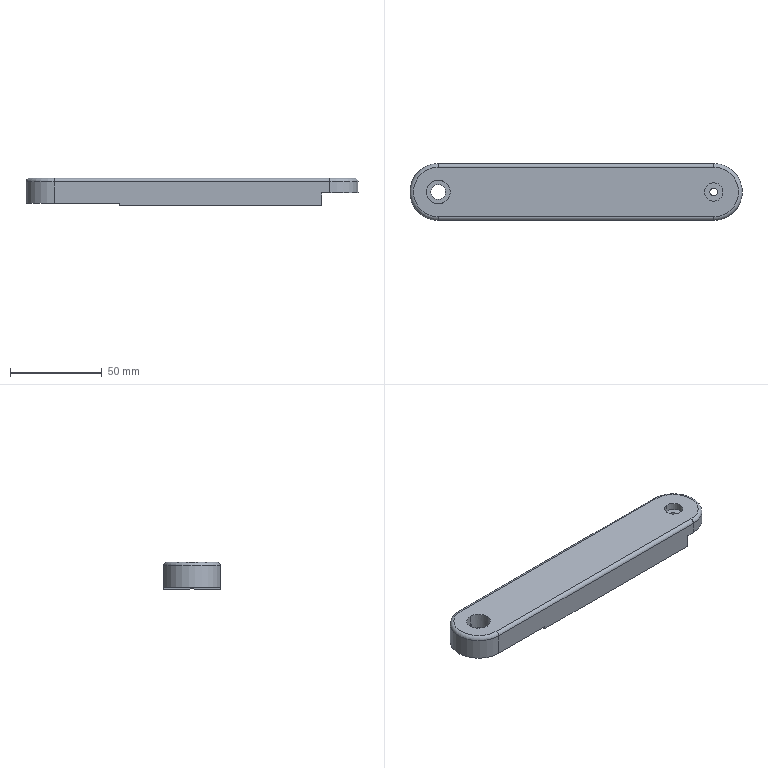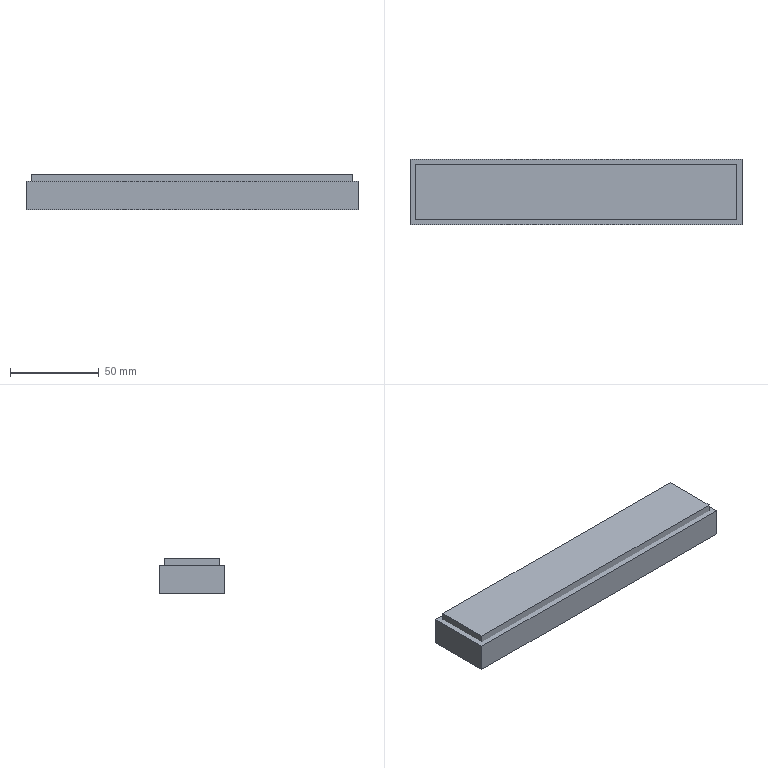CAM job | NX | 3-axis milling, drilling | part box 181 x 31 x 15 mm | stock box 187 x 37 x 20 mm
Tools:
number,name,description,diameter,corner_radius,flute_length,length,flutes
19,D80,Milling Tool-5 Parameters,80.0,0.0,50.0,75.0,2
1,D6A45,Milling Tool-5 Parameters,6.0,0.0,50.0,75.0,2
2,2.1ZT,Drilling Tool,2.05,0.0,35.0,50.0,2
16,1.6ZT,Drilling Tool,1.6,0.0,35.0,50.0,2
24,1.5ZT,Drilling Tool,1.5,0.0,35.0,50.0,2
4,4.2ZT,Drilling Tool,4.2,0.0,35.0,50.0,2
15,D10,Milling Tool-5 Parameters,10.0,0.0,50.0,75.0,2
14,D10JING,Milling Tool-5 Parameters,10.0,0.0,50.0,75.0,2
12,D6,Milling Tool-5 Parameters,6.0,0.0,50.0,75.0,2
17,D2,Milling Tool-5 Parameters,2.0,0.0,50.0,75.0,2
11,D4,Milling Tool-5 Parameters,4.0,0.0,50.0,75.0,2
21,R2,Milling Tool-5 Parameters,4.0,2.0,50.0,75.0,2
18,D6R0.5,Milling Tool-5 Parameters,6.0,0.5,50.0,75.0,2
Operations:
program,operation,operation_type,tool,method,geometry_group,spindle_rpm,surface_speed,feed_per_tooth,feed_cut,feed_plunge,cut_length_mm,path_length_mm,cut_time_min,machine_time_min
1,FLOOR_WALL_COPY,VolumeBased25DMillingOperation,D80,METHOD,A,6500.0,1633.0,0.1154,1500.0,100.0,283.0,337.0,0.1887,0.1941
1,DRILLING_COPY_1,Operation,D6A45,METHOD,A,5000.0,94.0,0.035,350.0,0.0,32.0,352.12,0.0914,0.1234
1,DRILLING_COPY_1_COPY,Operation,2.1ZT,METHOD,A,2000.0,12.0,0.0375,150.0,0.0,33.232,147.712,0.2215,0.233
1,DRILLING_COPY_1_COPY_COPY,Operation,1.6ZT,METHOD,A,2000.0,12.0,0.0375,150.0,0.0,39.923,210.521,0.2662,0.2832
1,DRILLING_COPY_1_COPY_COPY_COPY,Operation,1.5ZT,METHOD,A,2000.0,12.0,0.0375,150.0,0.0,51.003,232.681,0.34,0.3582
1,DRILLING_COPY_1_COPY_1,Operation,4.2ZT,METHOD,A,2000.0,34.0,0.05,200.0,0.0,20.262,100.524,0.1013,0.1093
1,ADAPTIVE_MILLING,CavityMilling,D10,METHOD,A,9500.0,298.0,0.1579,3000.0,1000.0,1947.53,2284.173,0.6532,0.6868
1,FLOOR_WALL,VolumeBased25DMillingOperation,D10,METHOD,A,9500.0,298.0,0.1316,2500.0,1000.0,1273.37,1440.847,0.5474,0.5641
1,FLOOR_WALL_COPY_1,VolumeBased25DMillingOperation,D10,METHOD,A,9500.0,298.0,0.1316,2500.0,1000.0,747.315,828.738,0.3098,0.318
1,ZLEVEL_PROFILE_COPY_1_COPY_COPY_1,ZLevelMilling,D10JING,METHOD,A,9500.0,298.0,0.0632,1200.0,1000.0,436.29,524.29,0.3642,0.373
1,FLOOR_WALL_1,VolumeBased25DMillingOperation,D10JING,METHOD,A,9500.0,298.0,0.0658,1250.0,100.0,676.572,1136.641,0.5413,0.5873
1,FLOOR_WALL_COPY_1_COPY,VolumeBased25DMillingOperation,D6,METHOD,A,9500.0,179.0,0.0868,1650.0,1000.0,1172.176,1259.534,0.7661,0.7748
1,FLOOR_WALL_1_COPY,VolumeBased25DMillingOperation,D6,METHOD,A,9500.0,298.0,0.0658,1250.0,100.0,364.716,558.998,0.2918,0.3112
1,HOLE_MILLING,CylinderMilling,D6,METHOD,A,9500.0,0.0,0.0,1650.0,100.0,270.469,431.069,0.1639,0.18
1,HOLE_MILLING_COPY,CylinderMilling,D4,METHOD,A,9500.0,0.0,0.0,1650.0,100.0,583.153,658.953,0.3534,0.361
1,ZLEVEL_PROFILE,ZLevelMilling,D2,METHOD,A,9500.0,59.0,0.0579,1100.0,100.0,348.462,844.207,0.3168,0.3664
1,FIXED_CONTOUR,SurfaceContour,R2,METHOD,A,9500.0,119.0,0.1316,2500.0,1000.0,1156.287,1209.887,0.465,0.4704
1,PLANAR_MILL_COPY_COPY_COPY_COPY_COPY_COPY_1_COPY_1,PlanarMilling,D6A45,METHOD,A,9500.0,179.0,0.0658,1250.0,100.0,298.924,357.924,0.2391,0.245
1,PLANAR_MILL_COPY_COPY_COPY_COPY_COPY_COPY_1_COPY_1_COPY,PlanarMilling,D6A45,METHOD,A,9500.0,179.0,0.0658,1250.0,100.0,92.815,413.435,0.0743,0.1063
1,PLANAR_MILL_COPY_COPY_COPY_COPY_COPY_COPY_1_COPY_1_COPY_COPY,PlanarMilling,D6A45,METHOD,A,9500.0,179.0,0.0658,1250.0,100.0,277.061,506.146,0.2216,0.2446
1,DRILLING_COPY_1_COPY_2,Operation,D6A45,METHOD,A,5000.0,94.0,0.035,350.0,0.0,28.35,337.279,0.081,0.1119
1,刀补11,CylinderMilling,D4,METHOD,A,9500.0,0.0,0.0526,1000.0,100.0,106.559,182.359,0.1066,0.1141
1,刀补12,CylinderMilling,D6,METHOD,A,9500.0,0.0,0.0526,1000.0,100.0,90.078,250.678,0.0901,0.1061
2,FLOOR_WALL_COPY_COPY,VolumeBased25DMillingOperation,D80,METHOD,B,6500.0,1633.0,0.1154,1500.0,100.0,1385.0,2719.001,0.9233,1.057
2,HOLE_MILLING_COPY_1,CylinderMilling,D6,METHOD,B,9500.0,0.0,0.0,1650.0,100.0,438.049,506.549,0.2655,0.2723
2,HOLE_MILLING_COPY_COPY,CylinderMilling,D4,METHOD,B,9500.0,0.0,0.0,1650.0,100.0,466.634,534.634,0.2828,0.2896
2,PLANAR_MILL_COPY_COPY_COPY_COPY_COPY_COPY_1_COPY_1_COPY_1,PlanarMilling,D6A45,METHOD,B,9500.0,179.0,0.0658,1250.0,100.0,77.073,347.985,0.0617,0.0887
2,ZLEVEL_PROFILE_1,ZLevelMilling,D6R0.5,METHOD,B,9500.0,119.0,0.1842,3500.0,100.0,15642.139,15698.648,4.469,4.475
2,刀补12_COPY,CylinderMilling,D6,METHOD,B,9500.0,0.0,0.0526,1000.0,100.0,135.987,204.487,0.136,0.1428